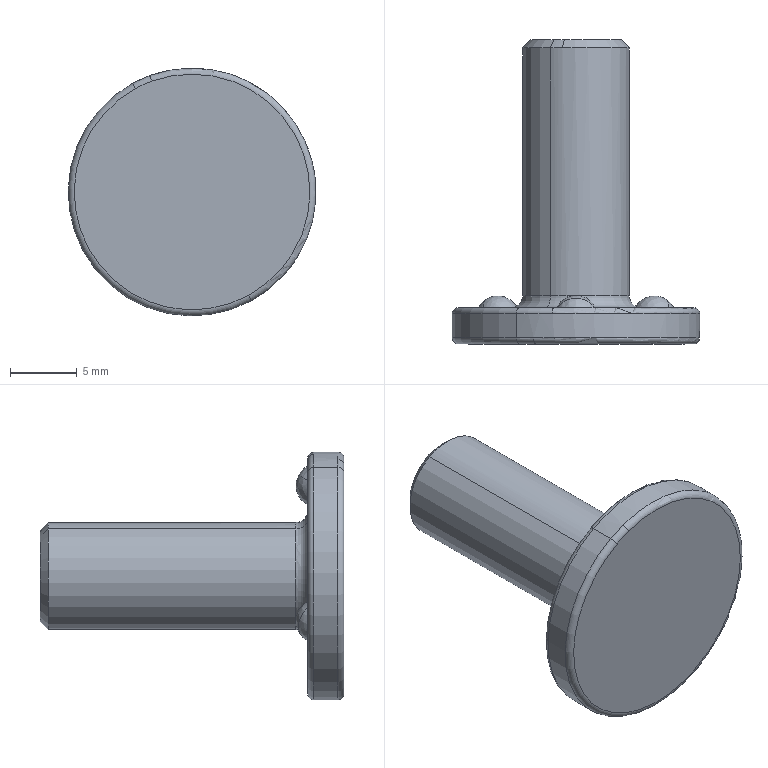Part | NX | features BREP 1 | 1 solid | 28 faces | box 18.5 x 22.7 x 18.5 mm | volume 1736 mm3 | torus 9 | sphere 9 | cylinder 4 | plane 3 | cone 3 | commonest cylinder face diameters 8 x2 18.5 x2